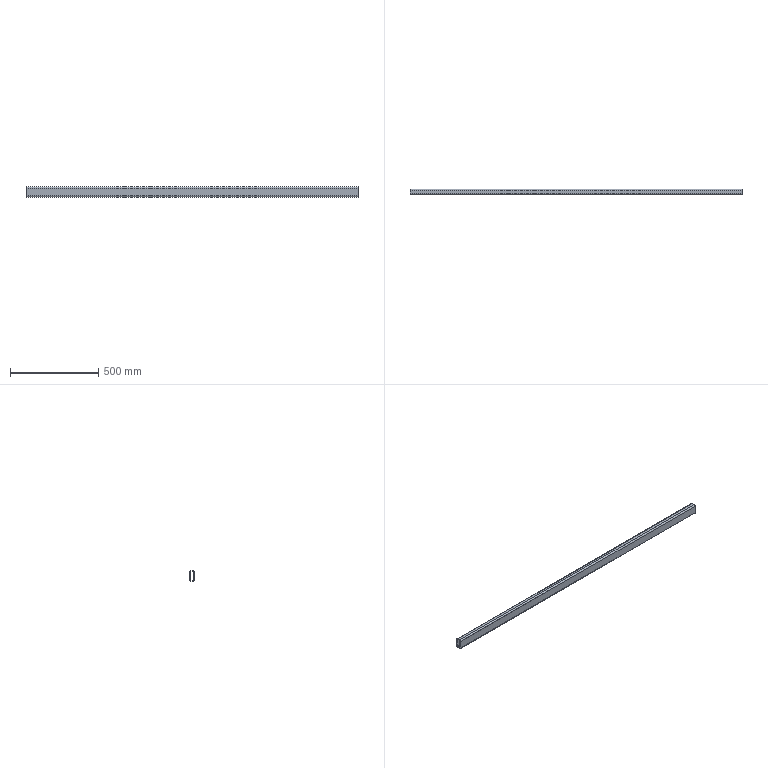Part | STEP file | 02-Rectangular tube 60x30x4_default<machining> | 1 solid | 18 faces | box 1880 x 30 x 60 mm | volume 1155817 mm3 | plane 10 | cylinder 8 | commonest cylinder face diameters 8 x4 16 x4
STEP:
#1=CARTESIAN_POINT('',(0.,0.,0.));
#2=DIRECTION('',(0.,0.,1.));
#3=DIRECTION('',(1.,0.,0.));
#4=AXIS2_PLACEMENT_3D('',#1,#2,#3);
#5=CARTESIAN_POINT('',(0.,15.,22.));
#6=VERTEX_POINT('',#5);
#7=CARTESIAN_POINT('',(0.,7.,30.));
#8=VERTEX_POINT('',#7);
#9=CARTESIAN_POINT('',(0.,7.,22.));
#10=DIRECTION('',(1.,0.,0.));
#11=DIRECTION('',(0.,0.,-1.));
#12=AXIS2_PLACEMENT_3D('',#9,#10,#11);
#13=CIRCLE('',#12,8.);
#14=CARTESIAN_POINT('',(1880.,7.,22.));
#15=DIRECTION('',(-1.,0.,0.));
#16=DIRECTION('',(0.,0.,1.));
#17=AXIS2_PLACEMENT_3D('',#14,#15,#16);
#18=CYLINDRICAL_SURFACE('',#17,8.);
#19=CARTESIAN_POINT('',(3.142,1880.));
#20=DIRECTION('',(-1.,0.));
#21=VECTOR('',#20,1.);
#22=LINE('',#19,#21);
#23=(GEOMETRIC_REPRESENTATION_CONTEXT(2)PARAMETRIC_REPRESENTATION_CONTEXT()REPRESENTATION_CONTEXT('',''));
#24=DEFINITIONAL_REPRESENTATION('',(#22),#23);
#25=PCURVE('',#18,#24);
#26=CARTESIAN_POINT('',(0.,7.,22.));
#27=DIRECTION('',(1.,0.,0.));
#28=DIRECTION('',(0.,0.,-1.));
#29=AXIS2_PLACEMENT_3D('',#26,#27,#28);
#30=PLANE('',#29);
#31=CARTESIAN_POINT('',(0.,0.));
#32=DIRECTION('',(1.,0.));
#33=AXIS2_PLACEMENT_2D('',#31,#32);
#34=CIRCLE('',#33,8.);
#35=(GEOMETRIC_REPRESENTATION_CONTEXT(2)PARAMETRIC_REPRESENTATION_CONTEXT()REPRESENTATION_CONTEXT('',''));
#36=DEFINITIONAL_REPRESENTATION('',(#34),#35);
#37=PCURVE('',#30,#36);
#38=SURFACE_CURVE('',#13,(#25,#37),.PCURVE_S1.);
#39=EDGE_CURVE('',#6,#8,#38,.T.);
#40=ORIENTED_EDGE('',*,*,#39,.T.);
#41=CARTESIAN_POINT('',(1880.,7.,30.));
#42=VERTEX_POINT('',#41);
#43=CARTESIAN_POINT('',(1880.,7.,30.));
#44=DIRECTION('',(-1.,0.,0.));
#45=VECTOR('',#44,1.);
#46=LINE('',#43,#45);
#47=CARTESIAN_POINT('',(0.,0.));
#48=DIRECTION('',(0.,1.));
#49=VECTOR('',#48,1.);
#50=LINE('',#47,#49);
#51=(GEOMETRIC_REPRESENTATION_CONTEXT(2)PARAMETRIC_REPRESENTATION_CONTEXT()REPRESENTATION_CONTEXT('',''));
#52=DEFINITIONAL_REPRESENTATION('',(#50),#51);
#53=PCURVE('',#18,#52);
#54=CARTESIAN_POINT('',(1880.,7.,30.));
#55=DIRECTION('',(0.,0.,-1.));
#56=DIRECTION('',(-1.,0.,0.));
#57=AXIS2_PLACEMENT_3D('',#54,#55,#56);
#58=PLANE('',#57);
#59=CARTESIAN_POINT('',(0.,0.));
#60=DIRECTION('',(1.,0.));
#61=VECTOR('',#60,1.);
#62=LINE('',#59,#61);
#63=(GEOMETRIC_REPRESENTATION_CONTEXT(2)PARAMETRIC_REPRESENTATION_CONTEXT()REPRESENTATION_CONTEXT('',''));
#64=DEFINITIONAL_REPRESENTATION('',(#62),#63);
#65=PCURVE('',#58,#64);
#66=SURFACE_CURVE('',#46,(#53,#65),.PCURVE_S1.);
#67=EDGE_CURVE('',#42,#8,#66,.T.);
#68=ORIENTED_EDGE('',*,*,#67,.F.);
#69=CARTESIAN_POINT('',(1880.,15.,22.));
#70=VERTEX_POINT('',#69);
#71=CARTESIAN_POINT('',(1880.,7.,22.));
#72=DIRECTION('',(1.,0.,0.));
#73=DIRECTION('',(0.,0.,-1.));
#74=AXIS2_PLACEMENT_3D('',#71,#72,#73);
#75=CIRCLE('',#74,8.);
#76=CARTESIAN_POINT('',(3.142,0.));
#77=DIRECTION('',(-1.,0.));
#78=VECTOR('',#77,1.);
#79=LINE('',#76,#78);
#80=(GEOMETRIC_REPRESENTATION_CONTEXT(2)PARAMETRIC_REPRESENTATION_CONTEXT()REPRESENTATION_CONTEXT('',''));
#81=DEFINITIONAL_REPRESENTATION('',(#79),#80);
#82=PCURVE('',#18,#81);
#83=CARTESIAN_POINT('',(1880.,7.,22.));
#84=DIRECTION('',(1.,0.,0.));
#85=DIRECTION('',(0.,0.,-1.));
#86=AXIS2_PLACEMENT_3D('',#83,#84,#85);
#87=PLANE('',#86);
#88=CARTESIAN_POINT('',(0.,0.));
#89=DIRECTION('',(1.,0.));
#90=AXIS2_PLACEMENT_2D('',#88,#89);
#91=CIRCLE('',#90,8.);
#92=(GEOMETRIC_REPRESENTATION_CONTEXT(2)PARAMETRIC_REPRESENTATION_CONTEXT()REPRESENTATION_CONTEXT('',''));
#93=DEFINITIONAL_REPRESENTATION('',(#91),#92);
#94=PCURVE('',#87,#93);
#95=SURFACE_CURVE('',#75,(#82,#94),.PCURVE_S1.);
#96=EDGE_CURVE('',#70,#42,#95,.T.);
#97=ORIENTED_EDGE('',*,*,#96,.F.);
#98=CARTESIAN_POINT('',(1880.,15.,22.));
#99=DIRECTION('',(-1.,0.,0.));
#100=VECTOR('',#99,1.);
#101=LINE('',#98,#100);
#102=CARTESIAN_POINT('',(1.571,0.));
#103=DIRECTION('',(0.,1.));
#104=VECTOR('',#103,1.);
#105=LINE('',#102,#104);
#106=(GEOMETRIC_REPRESENTATION_CONTEXT(2)PARAMETRIC_REPRESENTATION_CONTEXT()REPRESENTATION_CONTEXT('',''));
#107=DEFINITIONAL_REPRESENTATION('',(#105),#106);
#108=PCURVE('',#18,#107);
#109=CARTESIAN_POINT('',(1880.,15.,22.));
#110=DIRECTION('',(0.,-1.,0.));
#111=DIRECTION('',(0.,0.,-1.));
#112=AXIS2_PLACEMENT_3D('',#109,#110,#111);
#113=PLANE('',#112);
#114=CARTESIAN_POINT('',(0.,0.));
#115=DIRECTION('',(0.,-1.));
#116=VECTOR('',#115,1.);
#117=LINE('',#114,#116);
#118=(GEOMETRIC_REPRESENTATION_CONTEXT(2)PARAMETRIC_REPRESENTATION_CONTEXT()REPRESENTATION_CONTEXT('',''));
#119=DEFINITIONAL_REPRESENTATION('',(#117),#118);
#120=PCURVE('',#113,#119);
#121=SURFACE_CURVE('',#101,(#108,#120),.PCURVE_S1.);
#122=EDGE_CURVE('',#70,#6,#121,.T.);
#123=ORIENTED_EDGE('',*,*,#122,.T.);
#124=EDGE_LOOP('',(#40,#68,#97,#123));
#125=FACE_BOUND('',#124,.T.);
#126=ADVANCED_FACE('',(#125),#18,.T.);
#127=CARTESIAN_POINT('',(0.,-7.,30.));
#128=VERTEX_POINT('',#127);
#129=CARTESIAN_POINT('',(0.,7.,30.));
#130=DIRECTION('',(0.,-1.,0.));
#131=VECTOR('',#130,1.);
#132=LINE('',#129,#131);
#133=CARTESIAN_POINT('',(1880.,0.));
#134=DIRECTION('',(0.,-1.));
#135=VECTOR('',#134,1.);
#136=LINE('',#133,#135);
#137=(GEOMETRIC_REPRESENTATION_CONTEXT(2)PARAMETRIC_REPRESENTATION_CONTEXT()REPRESENTATION_CONTEXT('',''));
#138=DEFINITIONAL_REPRESENTATION('',(#136),#137);
#139=PCURVE('',#58,#138);
#140=CARTESIAN_POINT('',(-8.,0.));
#141=DIRECTION('',(0.,-1.));
#142=VECTOR('',#141,1.);
#143=LINE('',#140,#142);
#144=(GEOMETRIC_REPRESENTATION_CONTEXT(2)PARAMETRIC_REPRESENTATION_CONTEXT()REPRESENTATION_CONTEXT('',''));
#145=DEFINITIONAL_REPRESENTATION('',(#143),#144);
#146=PCURVE('',#30,#145);
#147=SURFACE_CURVE('',#132,(#139,#146),.PCURVE_S1.);
#148=EDGE_CURVE('',#8,#128,#147,.T.);
#149=ORIENTED_EDGE('',*,*,#148,.T.);
#150=CARTESIAN_POINT('',(1880.,-7.,30.));
#151=VERTEX_POINT('',#150);
#152=CARTESIAN_POINT('',(1880.,-7.,30.));
#153=DIRECTION('',(-1.,0.,0.));
#154=VECTOR('',#153,1.);
#155=LINE('',#152,#154);
#156=CARTESIAN_POINT('',(0.,-14.));
#157=DIRECTION('',(1.,0.));
#158=VECTOR('',#157,1.);
#159=LINE('',#156,#158);
#160=(GEOMETRIC_REPRESENTATION_CONTEXT(2)PARAMETRIC_REPRESENTATION_CONTEXT()REPRESENTATION_CONTEXT('',''));
#161=DEFINITIONAL_REPRESENTATION('',(#159),#160);
#162=PCURVE('',#58,#161);
#163=CARTESIAN_POINT('',(1880.,-7.,22.));
#164=DIRECTION('',(-1.,0.,0.));
#165=DIRECTION('',(0.,0.,1.));
#166=AXIS2_PLACEMENT_3D('',#163,#164,#165);
#167=CYLINDRICAL_SURFACE('',#166,8.);
#168=CARTESIAN_POINT('',(6.283,0.));
#169=DIRECTION('',(0.,1.));
#170=VECTOR('',#169,1.);
#171=LINE('',#168,#170);
#172=(GEOMETRIC_REPRESENTATION_CONTEXT(2)PARAMETRIC_REPRESENTATION_CONTEXT()REPRESENTATION_CONTEXT('',''));
#173=DEFINITIONAL_REPRESENTATION('',(#171),#172);
#174=PCURVE('',#167,#173);
#175=SURFACE_CURVE('',#155,(#162,#174),.PCURVE_S1.);
#176=EDGE_CURVE('',#151,#128,#175,.T.);
#177=ORIENTED_EDGE('',*,*,#176,.F.);
#178=CARTESIAN_POINT('',(1880.,7.,30.));
#179=DIRECTION('',(0.,-1.,0.));
#180=VECTOR('',#179,1.);
#181=LINE('',#178,#180);
#182=CARTESIAN_POINT('',(0.,0.));
#183=DIRECTION('',(0.,-1.));
#184=VECTOR('',#183,1.);
#185=LINE('',#182,#184);
#186=(GEOMETRIC_REPRESENTATION_CONTEXT(2)PARAMETRIC_REPRESENTATION_CONTEXT()REPRESENTATION_CONTEXT('',''));
#187=DEFINITIONAL_REPRESENTATION('',(#185),#186);
#188=PCURVE('',#58,#187);
#189=CARTESIAN_POINT('',(-8.,0.));
#190=DIRECTION('',(0.,-1.));
#191=VECTOR('',#190,1.);
#192=LINE('',#189,#191);
#193=(GEOMETRIC_REPRESENTATION_CONTEXT(2)PARAMETRIC_REPRESENTATION_CONTEXT()REPRESENTATION_CONTEXT('',''));
#194=DEFINITIONAL_REPRESENTATION('',(#192),#193);
#195=PCURVE('',#87,#194);
#196=SURFACE_CURVE('',#181,(#188,#195),.PCURVE_S1.);
#197=EDGE_CURVE('',#42,#151,#196,.T.);
#198=ORIENTED_EDGE('',*,*,#197,.F.);
#199=ORIENTED_EDGE('',*,*,#67,.T.);
#200=EDGE_LOOP('',(#149,#177,#198,#199));
#201=FACE_BOUND('',#200,.T.);
#202=ADVANCED_FACE('',(#201),#58,.F.);
#203=CARTESIAN_POINT('',(0.,-15.,22.));
#204=VERTEX_POINT('',#203);
#205=CARTESIAN_POINT('',(0.,-7.,22.));
#206=DIRECTION('',(1.,0.,0.));
#207=DIRECTION('',(0.,0.,-1.));
#208=AXIS2_PLACEMENT_3D('',#205,#206,#207);
#209=CIRCLE('',#208,8.);
#210=CARTESIAN_POINT('',(9.425,1880.));
#211=DIRECTION('',(-1.,0.));
#212=VECTOR('',#211,1.);
#213=LINE('',#210,#212);
#214=(GEOMETRIC_REPRESENTATION_CONTEXT(2)PARAMETRIC_REPRESENTATION_CONTEXT()REPRESENTATION_CONTEXT('',''));
#215=DEFINITIONAL_REPRESENTATION('',(#213),#214);
#216=PCURVE('',#167,#215);
#217=CARTESIAN_POINT('',(0.,-14.));
#218=DIRECTION('',(1.,0.));
#219=AXIS2_PLACEMENT_2D('',#217,#218);
#220=CIRCLE('',#219,8.);
#221=(GEOMETRIC_REPRESENTATION_CONTEXT(2)PARAMETRIC_REPRESENTATION_CONTEXT()REPRESENTATION_CONTEXT('',''));
#222=DEFINITIONAL_REPRESENTATION('',(#220),#221);
#223=PCURVE('',#30,#222);
#224=SURFACE_CURVE('',#209,(#216,#223),.PCURVE_S1.);
#225=EDGE_CURVE('',#128,#204,#224,.T.);
#226=ORIENTED_EDGE('',*,*,#225,.T.);
#227=CARTESIAN_POINT('',(1880.,-15.,22.));
#228=VERTEX_POINT('',#227);
#229=CARTESIAN_POINT('',(1880.,-15.,22.));
#230=DIRECTION('',(-1.,0.,0.));
#231=VECTOR('',#230,1.);
#232=LINE('',#229,#231);
#233=CARTESIAN_POINT('',(4.712,0.));
#234=DIRECTION('',(0.,1.));
#235=VECTOR('',#234,1.);
#236=LINE('',#233,#235);
#237=(GEOMETRIC_REPRESENTATION_CONTEXT(2)PARAMETRIC_REPRESENTATION_CONTEXT()REPRESENTATION_CONTEXT('',''));
#238=DEFINITIONAL_REPRESENTATION('',(#236),#237);
#239=PCURVE('',#167,#238);
#240=CARTESIAN_POINT('',(1880.,-15.,-22.));
#241=DIRECTION('',(0.,1.,0.));
#242=DIRECTION('',(0.,0.,1.));
#243=AXIS2_PLACEMENT_3D('',#240,#241,#242);
#244=PLANE('',#243);
#245=CARTESIAN_POINT('',(44.,0.));
#246=DIRECTION('',(0.,-1.));
#247=VECTOR('',#246,1.);
#248=LINE('',#245,#247);
#249=(GEOMETRIC_REPRESENTATION_CONTEXT(2)PARAMETRIC_REPRESENTATION_CONTEXT()REPRESENTATION_CONTEXT('',''));
#250=DEFINITIONAL_REPRESENTATION('',(#248),#249);
#251=PCURVE('',#244,#250);
#252=SURFACE_CURVE('',#232,(#239,#251),.PCURVE_S1.);
#253=EDGE_CURVE('',#228,#204,#252,.T.);
#254=ORIENTED_EDGE('',*,*,#253,.F.);
#255=CARTESIAN_POINT('',(1880.,-7.,22.));
#256=DIRECTION('',(1.,0.,0.));
#257=DIRECTION('',(0.,0.,-1.));
#258=AXIS2_PLACEMENT_3D('',#255,#256,#257);
#259=CIRCLE('',#258,8.);
#260=CARTESIAN_POINT('',(9.425,0.));
#261=DIRECTION('',(-1.,0.));
#262=VECTOR('',#261,1.);
#263=LINE('',#260,#262);
#264=(GEOMETRIC_REPRESENTATION_CONTEXT(2)PARAMETRIC_REPRESENTATION_CONTEXT()REPRESENTATION_CONTEXT('',''));
#265=DEFINITIONAL_REPRESENTATION('',(#263),#264);
#266=PCURVE('',#167,#265);
#267=CARTESIAN_POINT('',(0.,-14.));
#268=DIRECTION('',(1.,0.));
#269=AXIS2_PLACEMENT_2D('',#267,#268);
#270=CIRCLE('',#269,8.);
#271=(GEOMETRIC_REPRESENTATION_CONTEXT(2)PARAMETRIC_REPRESENTATION_CONTEXT()REPRESENTATION_CONTEXT('',''));
#272=DEFINITIONAL_REPRESENTATION('',(#270),#271);
#273=PCURVE('',#87,#272);
#274=SURFACE_CURVE('',#259,(#266,#273),.PCURVE_S1.);
#275=EDGE_CURVE('',#151,#228,#274,.T.);
#276=ORIENTED_EDGE('',*,*,#275,.F.);
#277=ORIENTED_EDGE('',*,*,#176,.T.);
#278=EDGE_LOOP('',(#226,#254,#276,#277));
#279=FACE_BOUND('',#278,.T.);
#280=ADVANCED_FACE('',(#279),#167,.T.);
#281=CARTESIAN_POINT('',(0.,-15.,-22.));
#282=VERTEX_POINT('',#281);
#283=CARTESIAN_POINT('',(0.,-15.,-22.));
#284=DIRECTION('',(0.,0.,-1.));
#285=VECTOR('',#284,1.);
#286=LINE('',#283,#285);
#287=CARTESIAN_POINT('',(0.,-1880.));
#288=DIRECTION('',(-1.,0.));
#289=VECTOR('',#288,1.);
#290=LINE('',#287,#289);
#291=(GEOMETRIC_REPRESENTATION_CONTEXT(2)PARAMETRIC_REPRESENTATION_CONTEXT()REPRESENTATION_CONTEXT('',''));
#292=DEFINITIONAL_REPRESENTATION('',(#290),#291);
#293=PCURVE('',#244,#292);
#294=CARTESIAN_POINT('',(44.,-22.));
#295=DIRECTION('',(1.,0.));
#296=VECTOR('',#295,1.);
#297=LINE('',#294,#296);
#298=(GEOMETRIC_REPRESENTATION_CONTEXT(2)PARAMETRIC_REPRESENTATION_CONTEXT()REPRESENTATION_CONTEXT('',''));
#299=DEFINITIONAL_REPRESENTATION('',(#297),#298);
#300=PCURVE('',#30,#299);
#301=SURFACE_CURVE('',#286,(#293,#300),.PCURVE_S1.);
#302=EDGE_CURVE('',#204,#282,#301,.T.);
#303=ORIENTED_EDGE('',*,*,#302,.T.);
#304=CARTESIAN_POINT('',(1880.,-15.,-22.));
#305=VERTEX_POINT('',#304);
#306=CARTESIAN_POINT('',(1880.,-15.,-22.));
#307=DIRECTION('',(-1.,0.,0.));
#308=VECTOR('',#307,1.);
#309=LINE('',#306,#308);
#310=CARTESIAN_POINT('',(0.,0.));
#311=DIRECTION('',(0.,-1.));
#312=VECTOR('',#311,1.);
#313=LINE('',#310,#312);
#314=(GEOMETRIC_REPRESENTATION_CONTEXT(2)PARAMETRIC_REPRESENTATION_CONTEXT()REPRESENTATION_CONTEXT('',''));
#315=DEFINITIONAL_REPRESENTATION('',(#313),#314);
#316=PCURVE('',#244,#315);
#317=CARTESIAN_POINT('',(1880.,-7.,-22.));
#318=DIRECTION('',(-1.,0.,0.));
#319=DIRECTION('',(0.,0.,1.));
#320=AXIS2_PLACEMENT_3D('',#317,#318,#319);
#321=CYLINDRICAL_SURFACE('',#320,8.);
#322=CARTESIAN_POINT('',(4.712,0.));
#323=DIRECTION('',(0.,1.));
#324=VECTOR('',#323,1.);
#325=LINE('',#322,#324);
#326=(GEOMETRIC_REPRESENTATION_CONTEXT(2)PARAMETRIC_REPRESENTATION_CONTEXT()REPRESENTATION_CONTEXT('',''));
#327=DEFINITIONAL_REPRESENTATION('',(#325),#326);
#328=PCURVE('',#321,#327);
#329=SURFACE_CURVE('',#309,(#316,#328),.PCURVE_S1.);
#330=EDGE_CURVE('',#305,#282,#329,.T.);
#331=ORIENTED_EDGE('',*,*,#330,.F.);
#332=CARTESIAN_POINT('',(1880.,-15.,-22.));
#333=DIRECTION('',(0.,0.,-1.));
#334=VECTOR('',#333,1.);
#335=LINE('',#332,#334);
#336=CARTESIAN_POINT('',(0.,0.));
#337=DIRECTION('',(-1.,0.));
#338=VECTOR('',#337,1.);
#339=LINE('',#336,#338);
#340=(GEOMETRIC_REPRESENTATION_CONTEXT(2)PARAMETRIC_REPRESENTATION_CONTEXT()REPRESENTATION_CONTEXT('',''));
#341=DEFINITIONAL_REPRESENTATION('',(#339),#340);
#342=PCURVE('',#244,#341);
#343=CARTESIAN_POINT('',(44.,-22.));
#344=DIRECTION('',(1.,0.));
#345=VECTOR('',#344,1.);
#346=LINE('',#343,#345);
#347=(GEOMETRIC_REPRESENTATION_CONTEXT(2)PARAMETRIC_REPRESENTATION_CONTEXT()REPRESENTATION_CONTEXT('',''));
#348=DEFINITIONAL_REPRESENTATION('',(#346),#347);
#349=PCURVE('',#87,#348);
#350=SURFACE_CURVE('',#335,(#342,#349),.PCURVE_S1.);
#351=EDGE_CURVE('',#228,#305,#350,.T.);
#352=ORIENTED_EDGE('',*,*,#351,.F.);
#353=ORIENTED_EDGE('',*,*,#253,.T.);
#354=EDGE_LOOP('',(#303,#331,#352,#353));
#355=FACE_BOUND('',#354,.T.);
#356=ADVANCED_FACE('',(#355),#244,.F.);
#357=CARTESIAN_POINT('',(0.,-7.,-30.));
#358=VERTEX_POINT('',#357);
#359=CARTESIAN_POINT('',(0.,-7.,-22.));
#360=DIRECTION('',(1.,0.,0.));
#361=DIRECTION('',(0.,0.,-1.));
#362=AXIS2_PLACEMENT_3D('',#359,#360,#361);
#363=CIRCLE('',#362,8.);
#364=CARTESIAN_POINT('',(9.425,1880.));
#365=DIRECTION('',(-1.,0.));
#366=VECTOR('',#365,1.);
#367=LINE('',#364,#366);
#368=(GEOMETRIC_REPRESENTATION_CONTEXT(2)PARAMETRIC_REPRESENTATION_CONTEXT()REPRESENTATION_CONTEXT('',''));
#369=DEFINITIONAL_REPRESENTATION('',(#367),#368);
#370=PCURVE('',#321,#369);
#371=CARTESIAN_POINT('',(44.,-14.));
#372=DIRECTION('',(1.,0.));
#373=AXIS2_PLACEMENT_2D('',#371,#372);
#374=CIRCLE('',#373,8.);
#375=(GEOMETRIC_REPRESENTATION_CONTEXT(2)PARAMETRIC_REPRESENTATION_CONTEXT()REPRESENTATION_CONTEXT('',''));
#376=DEFINITIONAL_REPRESENTATION('',(#374),#375);
#377=PCURVE('',#30,#376);
#378=SURFACE_CURVE('',#363,(#370,#377),.PCURVE_S1.);
#379=EDGE_CURVE('',#282,#358,#378,.T.);
#380=ORIENTED_EDGE('',*,*,#379,.T.);
#381=CARTESIAN_POINT('',(1880.,-7.,-30.));
#382=VERTEX_POINT('',#381);
#383=CARTESIAN_POINT('',(1880.,-7.,-30.));
#384=DIRECTION('',(-1.,0.,0.));
#385=VECTOR('',#384,1.);
#386=LINE('',#383,#385);
#387=CARTESIAN_POINT('',(3.142,0.));
#388=DIRECTION('',(0.,1.));
#389=VECTOR('',#388,1.);
#390=LINE('',#387,#389);
#391=(GEOMETRIC_REPRESENTATION_CONTEXT(2)PARAMETRIC_REPRESENTATION_CONTEXT()REPRESENTATION_CONTEXT('',''));
#392=DEFINITIONAL_REPRESENTATION('',(#390),#391);
#393=PCURVE('',#321,#392);
#394=CARTESIAN_POINT('',(1880.,-7.,-30.));
#395=DIRECTION('',(0.,0.,1.));
#396=DIRECTION('',(1.,0.,0.));
#397=AXIS2_PLACEMENT_3D('',#394,#395,#396);
#398=PLANE('',#397);
#399=CARTESIAN_POINT('',(0.,0.));
#400=DIRECTION('',(-1.,0.));
#401=VECTOR('',#400,1.);
#402=LINE('',#399,#401);
#403=(GEOMETRIC_REPRESENTATION_CONTEXT(2)PARAMETRIC_REPRESENTATION_CONTEXT()REPRESENTATION_CONTEXT('',''));
#404=DEFINITIONAL_REPRESENTATION('',(#402),#403);
#405=PCURVE('',#398,#404);
#406=SURFACE_CURVE('',#386,(#393,#405),.PCURVE_S1.);
#407=EDGE_CURVE('',#382,#358,#406,.T.);
#408=ORIENTED_EDGE('',*,*,#407,.F.);
#409=CARTESIAN_POINT('',(1880.,-7.,-22.));
#410=DIRECTION('',(1.,0.,0.));
#411=DIRECTION('',(0.,0.,-1.));
#412=AXIS2_PLACEMENT_3D('',#409,#410,#411);
#413=CIRCLE('',#412,8.);
#414=CARTESIAN_POINT('',(9.425,0.));
#415=DIRECTION('',(-1.,0.));
#416=VECTOR('',#415,1.);
#417=LINE('',#414,#416);
#418=(GEOMETRIC_REPRESENTATION_CONTEXT(2)PARAMETRIC_REPRESENTATION_CONTEXT()REPRESENTATION_CONTEXT('',''));
#419=DEFINITIONAL_REPRESENTATION('',(#417),#418);
#420=PCURVE('',#321,#419);
#421=CARTESIAN_POINT('',(44.,-14.));
#422=DIRECTION('',(1.,0.));
#423=AXIS2_PLACEMENT_2D('',#421,#422);
#424=CIRCLE('',#423,8.);
#425=(GEOMETRIC_REPRESENTATION_CONTEXT(2)PARAMETRIC_REPRESENTATION_CONTEXT()REPRESENTATION_CONTEXT('',''));
#426=DEFINITIONAL_REPRESENTATION('',(#424),#425);
#427=PCURVE('',#87,#426);
#428=SURFACE_CURVE('',#413,(#420,#427),.PCURVE_S1.);
#429=EDGE_CURVE('',#305,#382,#428,.T.);
#430=ORIENTED_EDGE('',*,*,#429,.F.);
#431=ORIENTED_EDGE('',*,*,#330,.T.);
#432=EDGE_LOOP('',(#380,#408,#430,#431));
#433=FACE_BOUND('',#432,.T.);
#434=ADVANCED_FACE('',(#433),#321,.T.);
#435=CARTESIAN_POINT('',(0.,7.,-30.));
#436=VERTEX_POINT('',#435);
#437=CARTESIAN_POINT('',(0.,-7.,-30.));
#438=DIRECTION('',(0.,1.,0.));
#439=VECTOR('',#438,1.);
#440=LINE('',#437,#439);
#441=CARTESIAN_POINT('',(-1880.,0.));
#442=DIRECTION('',(0.,1.));
#443=VECTOR('',#442,1.);
#444=LINE('',#441,#443);
#445=(GEOMETRIC_REPRESENTATION_CONTEXT(2)PARAMETRIC_REPRESENTATION_CONTEXT()REPRESENTATION_CONTEXT('',''));
#446=DEFINITIONAL_REPRESENTATION('',(#444),#445);
#447=PCURVE('',#398,#446);
#448=CARTESIAN_POINT('',(52.,-14.));
#449=DIRECTION('',(0.,1.));
#450=VECTOR('',#449,1.);
#451=LINE('',#448,#450);
#452=(GEOMETRIC_REPRESENTATION_CONTEXT(2)PARAMETRIC_REPRESENTATION_CONTEXT()REPRESENTATION_CONTEXT('',''));
#453=DEFINITIONAL_REPRESENTATION('',(#451),#452);
#454=PCURVE('',#30,#453);
#455=SURFACE_CURVE('',#440,(#447,#454),.PCURVE_S1.);
#456=EDGE_CURVE('',#358,#436,#455,.T.);
#457=ORIENTED_EDGE('',*,*,#456,.T.);
#458=CARTESIAN_POINT('',(1880.,7.,-30.));
#459=VERTEX_POINT('',#458);
#460=CARTESIAN_POINT('',(1880.,7.,-30.));
#461=DIRECTION('',(-1.,0.,0.));
#462=VECTOR('',#461,1.);
#463=LINE('',#460,#462);
#464=CARTESIAN_POINT('',(0.,14.));
#465=DIRECTION('',(-1.,0.));
#466=VECTOR('',#465,1.);
#467=LINE('',#464,#466);
#468=(GEOMETRIC_REPRESENTATION_CONTEXT(2)PARAMETRIC_REPRESENTATION_CONTEXT()REPRESENTATION_CONTEXT('',''));
#469=DEFINITIONAL_REPRESENTATION('',(#467),#468);
#470=PCURVE('',#398,#469);
#471=CARTESIAN_POINT('',(1880.,7.,-22.));
#472=DIRECTION('',(-1.,0.,0.));
#473=DIRECTION('',(0.,0.,1.));
#474=AXIS2_PLACEMENT_3D('',#471,#472,#473);
#475=CYLINDRICAL_SURFACE('',#474,8.);
#476=CARTESIAN_POINT('',(3.142,0.));
#477=DIRECTION('',(0.,1.));
#478=VECTOR('',#477,1.);
#479=LINE('',#476,#478);
#480=(GEOMETRIC_REPRESENTATION_CONTEXT(2)PARAMETRIC_REPRESENTATION_CONTEXT()REPRESENTATION_CONTEXT('',''));
#481=DEFINITIONAL_REPRESENTATION('',(#479),#480);
#482=PCURVE('',#475,#481);
#483=SURFACE_CURVE('',#463,(#470,#482),.PCURVE_S1.);
#484=EDGE_CURVE('',#459,#436,#483,.T.);
#485=ORIENTED_EDGE('',*,*,#484,.F.);
#486=CARTESIAN_POINT('',(1880.,-7.,-30.));
#487=DIRECTION('',(0.,1.,0.));
#488=VECTOR('',#487,1.);
#489=LINE('',#486,#488);
#490=CARTESIAN_POINT('',(0.,0.));
#491=DIRECTION('',(0.,1.));
#492=VECTOR('',#491,1.);
#493=LINE('',#490,#492);
#494=(GEOMETRIC_REPRESENTATION_CONTEXT(2)PARAMETRIC_REPRESENTATION_CONTEXT()REPRESENTATION_CONTEXT('',''));
#495=DEFINITIONAL_REPRESENTATION('',(#493),#494);
#496=PCURVE('',#398,#495);
#497=CARTESIAN_POINT('',(52.,-14.));
#498=DIRECTION('',(0.,1.));
#499=VECTOR('',#498,1.);
#500=LINE('',#497,#499);
#501=(GEOMETRIC_REPRESENTATION_CONTEXT(2)PARAMETRIC_REPRESENTATION_CONTEXT()REPRESENTATION_CONTEXT('',''));
#502=DEFINITIONAL_REPRESENTATION('',(#500),#501);
#503=PCURVE('',#87,#502);
#504=SURFACE_CURVE('',#489,(#496,#503),.PCURVE_S1.);
#505=EDGE_CURVE('',#382,#459,#504,.T.);
#506=ORIENTED_EDGE('',*,*,#505,.F.);
#507=ORIENTED_EDGE('',*,*,#407,.T.);
#508=EDGE_LOOP('',(#457,#485,#506,#507));
#509=FACE_BOUND('',#508,.T.);
#510=ADVANCED_FACE('',(#509),#398,.F.);
#511=CARTESIAN_POINT('',(0.,15.,-22.));
#512=VERTEX_POINT('',#511);
#513=CARTESIAN_POINT('',(0.,7.,-22.));
#514=DIRECTION('',(1.,0.,0.));
#515=DIRECTION('',(0.,0.,-1.));
#516=AXIS2_PLACEMENT_3D('',#513,#514,#515);
#517=CIRCLE('',#516,8.);
#518=CARTESIAN_POINT('',(3.142,1880.));
#519=DIRECTION('',(-1.,0.));
#520=VECTOR('',#519,1.);
#521=LINE('',#518,#520);
#522=(GEOMETRIC_REPRESENTATION_CONTEXT(2)PARAMETRIC_REPRESENTATION_CONTEXT()REPRESENTATION_CONTEXT('',''));
#523=DEFINITIONAL_REPRESENTATION('',(#521),#522);
#524=PCURVE('',#475,#523);
#525=CARTESIAN_POINT('',(44.,0.));
#526=DIRECTION('',(1.,0.));
#527=AXIS2_PLACEMENT_2D('',#525,#526);
#528=CIRCLE('',#527,8.);
#529=(GEOMETRIC_REPRESENTATION_CONTEXT(2)PARAMETRIC_REPRESENTATION_CONTEXT()REPRESENTATION_CONTEXT('',''));
#530=DEFINITIONAL_REPRESENTATION('',(#528),#529);
#531=PCURVE('',#30,#530);
#532=SURFACE_CURVE('',#517,(#524,#531),.PCURVE_S1.);
#533=EDGE_CURVE('',#436,#512,#532,.T.);
#534=ORIENTED_EDGE('',*,*,#533,.T.);
#535=CARTESIAN_POINT('',(1880.,15.,-22.));
#536=VERTEX_POINT('',#535);
#537=CARTESIAN_POINT('',(1880.,15.,-22.));
#538=DIRECTION('',(-1.,0.,0.));
#539=VECTOR('',#538,1.);
#540=LINE('',#537,#539);
#541=CARTESIAN_POINT('',(1.571,0.));
#542=DIRECTION('',(0.,1.));
#543=VECTOR('',#542,1.);
#544=LINE('',#541,#543);
#545=(GEOMETRIC_REPRESENTATION_CONTEXT(2)PARAMETRIC_REPRESENTATION_CONTEXT()REPRESENTATION_CONTEXT('',''));
#546=DEFINITIONAL_REPRESENTATION('',(#544),#545);
#547=PCURVE('',#475,#546);
#548=CARTESIAN_POINT('',(44.,0.));
#549=DIRECTION('',(0.,-1.));
#550=VECTOR('',#549,1.);
#551=LINE('',#548,#550);
#552=(GEOMETRIC_REPRESENTATION_CONTEXT(2)PARAMETRIC_REPRESENTATION_CONTEXT()REPRESENTATION_CONTEXT('',''));
#553=DEFINITIONAL_REPRESENTATION('',(#551),#552);
#554=PCURVE('',#113,#553);
#555=SURFACE_CURVE('',#540,(#547,#554),.PCURVE_S1.);
#556=EDGE_CURVE('',#536,#512,#555,.T.);
#557=ORIENTED_EDGE('',*,*,#556,.F.);
#558=CARTESIAN_POINT('',(1880.,7.,-22.));
#559=DIRECTION('',(1.,0.,0.));
#560=DIRECTION('',(0.,0.,-1.));
#561=AXIS2_PLACEMENT_3D('',#558,#559,#560);
#562=CIRCLE('',#561,8.);
#563=CARTESIAN_POINT('',(3.142,0.));
#564=DIRECTION('',(-1.,0.));
#565=VECTOR('',#564,1.);
#566=LINE('',#563,#565);
#567=(GEOMETRIC_REPRESENTATION_CONTEXT(2)PARAMETRIC_REPRESENTATION_CONTEXT()REPRESENTATION_CONTEXT('',''));
#568=DEFINITIONAL_REPRESENTATION('',(#566),#567);
#569=PCURVE('',#475,#568);
#570=CARTESIAN_POINT('',(44.,0.));
#571=DIRECTION('',(1.,0.));
#572=AXIS2_PLACEMENT_2D('',#570,#571);
#573=CIRCLE('',#572,8.);
#574=(GEOMETRIC_REPRESENTATION_CONTEXT(2)PARAMETRIC_REPRESENTATION_CONTEXT()REPRESENTATION_CONTEXT('',''));
#575=DEFINITIONAL_REPRESENTATION('',(#573),#574);
#576=PCURVE('',#87,#575);
#577=SURFACE_CURVE('',#562,(#569,#576),.PCURVE_S1.);
#578=EDGE_CURVE('',#459,#536,#577,.T.);
#579=ORIENTED_EDGE('',*,*,#578,.F.);
#580=ORIENTED_EDGE('',*,*,#484,.T.);
#581=EDGE_LOOP('',(#534,#557,#579,#580));
#582=FACE_BOUND('',#581,.T.);
#583=ADVANCED_FACE('',(#582),#475,.T.);
#584=CARTESIAN_POINT('',(1880.,-11.,22.));
#585=VERTEX_POINT('',#584);
#586=CARTESIAN_POINT('',(0.,-11.,22.));
#587=VERTEX_POINT('',#586);
#588=CARTESIAN_POINT('',(1880.,-11.,22.));
#589=DIRECTION('',(-1.,0.,0.));
#590=VECTOR('',#589,1.);
#591=LINE('',#588,#590);
#592=CARTESIAN_POINT('',(1880.,-7.,22.));
#593=DIRECTION('',(-1.,0.,0.));
#594=DIRECTION('',(0.,0.,1.));
#595=AXIS2_PLACEMENT_3D('',#592,#593,#594);
#596=CYLINDRICAL_SURFACE('',#595,4.);
#597=CARTESIAN_POINT('',(4.712,0.));
#598=DIRECTION('',(0.,1.));
#599=VECTOR('',#598,1.);
#600=LINE('',#597,#599);
#601=(GEOMETRIC_REPRESENTATION_CONTEXT(2)PARAMETRIC_REPRESENTATION_CONTEXT()REPRESENTATION_CONTEXT('',''));
#602=DEFINITIONAL_REPRESENTATION('',(#600),#601);
#603=PCURVE('',#596,#602);
#604=CARTESIAN_POINT('',(1880.,-11.,-22.));
#605=DIRECTION('',(0.,1.,0.));
#606=DIRECTION('',(0.,0.,1.));
#607=AXIS2_PLACEMENT_3D('',#604,#605,#606);
#608=PLANE('',#607);
#609=CARTESIAN_POINT('',(44.,0.));
#610=DIRECTION('',(0.,-1.));
#611=VECTOR('',#610,1.);
#612=LINE('',#609,#611);
#613=(GEOMETRIC_REPRESENTATION_CONTEXT(2)PARAMETRIC_REPRESENTATION_CONTEXT()REPRESENTATION_CONTEXT('',''));
#614=DEFINITIONAL_REPRESENTATION('',(#612),#613);
#615=PCURVE('',#608,#614);
#616=SURFACE_CURVE('',#591,(#603,#615),.PCURVE_S1.);
#617=EDGE_CURVE('',#585,#587,#616,.T.);
#618=ORIENTED_EDGE('',*,*,#617,.F.);
#619=CARTESIAN_POINT('',(1880.,-7.,26.));
#620=VERTEX_POINT('',#619);
#621=CARTESIAN_POINT('',(1880.,-7.,22.));
#622=DIRECTION('',(1.,0.,0.));
#623=DIRECTION('',(0.,0.,-1.));
#624=AXIS2_PLACEMENT_3D('',#621,#622,#623);
#625=CIRCLE('',#624,4.);
#626=CARTESIAN_POINT('',(9.425,0.));
#627=DIRECTION('',(-1.,0.));
#628=VECTOR('',#627,1.);
#629=LINE('',#626,#628);
#630=(GEOMETRIC_REPRESENTATION_CONTEXT(2)PARAMETRIC_REPRESENTATION_CONTEXT()REPRESENTATION_CONTEXT('',''));
#631=DEFINITIONAL_REPRESENTATION('',(#629),#630);
#632=PCURVE('',#596,#631);
#633=CARTESIAN_POINT('',(0.,-14.));
#634=DIRECTION('',(1.,0.));
#635=AXIS2_PLACEMENT_2D('',#633,#634);
#636=CIRCLE('',#635,4.);
#637=(GEOMETRIC_REPRESENTATION_CONTEXT(2)PARAMETRIC_REPRESENTATION_CONTEXT()REPRESENTATION_CONTEXT('',''));
#638=DEFINITIONAL_REPRESENTATION('',(#636),#637);
#639=PCURVE('',#87,#638);
#640=SURFACE_CURVE('',#625,(#632,#639),.PCURVE_S1.);
#641=EDGE_CURVE('',#620,#585,#640,.T.);
#642=ORIENTED_EDGE('',*,*,#641,.F.);
#643=CARTESIAN_POINT('',(0.,-7.,26.));
#644=VERTEX_POINT('',#643);
#645=CARTESIAN_POINT('',(1880.,-7.,26.));
#646=DIRECTION('',(-1.,0.,0.));
#647=VECTOR('',#646,1.);
#648=LINE('',#645,#647);
#649=CARTESIAN_POINT('',(6.283,0.));
#650=DIRECTION('',(0.,1.));
#651=VECTOR('',#650,1.);
#652=LINE('',#649,#651);
#653=(GEOMETRIC_REPRESENTATION_CONTEXT(2)PARAMETRIC_REPRESENTATION_CONTEXT()REPRESENTATION_CONTEXT('',''));
#654=DEFINITIONAL_REPRESENTATION('',(#652),#653);
#655=PCURVE('',#596,#654);
#656=CARTESIAN_POINT('',(1880.,7.,26.));
#657=DIRECTION('',(0.,0.,-1.));
#658=DIRECTION('',(-1.,0.,0.));
#659=AXIS2_PLACEMENT_3D('',#656,#657,#658);
#660=PLANE('',#659);
#661=CARTESIAN_POINT('',(0.,-14.));
#662=DIRECTION('',(1.,0.));
#663=VECTOR('',#662,1.);
#664=LINE('',#661,#663);
#665=(GEOMETRIC_REPRESENTATION_CONTEXT(2)PARAMETRIC_REPRESENTATION_CONTEXT()REPRESENTATION_CONTEXT('',''));
#666=DEFINITIONAL_REPRESENTATION('',(#664),#665);
#667=PCURVE('',#660,#666);
#668=SURFACE_CURVE('',#648,(#655,#667),.PCURVE_S1.);
#669=EDGE_CURVE('',#620,#644,#668,.T.);
#670=ORIENTED_EDGE('',*,*,#669,.T.);
#671=CARTESIAN_POINT('',(0.,-7.,22.));
#672=DIRECTION('',(1.,0.,0.));
#673=DIRECTION('',(0.,0.,-1.));
#674=AXIS2_PLACEMENT_3D('',#671,#672,#673);
#675=CIRCLE('',#674,4.);
#676=CARTESIAN_POINT('',(9.425,1880.));
#677=DIRECTION('',(-1.,0.));
#678=VECTOR('',#677,1.);
#679=LINE('',#676,#678);
#680=(GEOMETRIC_REPRESENTATION_CONTEXT(2)PARAMETRIC_REPRESENTATION_CONTEXT()REPRESENTATION_CONTEXT('',''));
#681=DEFINITIONAL_REPRESENTATION('',(#679),#680);
#682=PCURVE('',#596,#681);
#683=CARTESIAN_POINT('',(0.,-14.));
#684=DIRECTION('',(1.,0.));
#685=AXIS2_PLACEMENT_2D('',#683,#684);
#686=CIRCLE('',#685,4.);
#687=(GEOMETRIC_REPRESENTATION_CONTEXT(2)PARAMETRIC_REPRESENTATION_CONTEXT()REPRESENTATION_CONTEXT('',''));
#688=DEFINITIONAL_REPRESENTATION('',(#686),#687);
#689=PCURVE('',#30,#688);
#690=SURFACE_CURVE('',#675,(#682,#689),.PCURVE_S1.);
#691=EDGE_CURVE('',#644,#587,#690,.T.);
#692=ORIENTED_EDGE('',*,*,#691,.T.);
#693=EDGE_LOOP('',(#618,#642,#670,#692));
#694=FACE_BOUND('',#693,.F.);
#695=ADVANCED_FACE('',(#694),#596,.F.);
#696=CARTESIAN_POINT('',(0.,7.,26.));
#697=VERTEX_POINT('',#696);
#698=CARTESIAN_POINT('',(0.,7.,26.));
#699=DIRECTION('',(0.,-1.,0.));
#700=VECTOR('',#699,1.);
#701=LINE('',#698,#700);
#702=CARTESIAN_POINT('',(1880.,0.));
#703=DIRECTION('',(0.,-1.));
#704=VECTOR('',#703,1.);
#705=LINE('',#702,#704);
#706=(GEOMETRIC_REPRESENTATION_CONTEXT(2)PARAMETRIC_REPRESENTATION_CONTEXT()REPRESENTATION_CONTEXT('',''));
#707=DEFINITIONAL_REPRESENTATION('',(#705),#706);
#708=PCURVE('',#660,#707);
#709=CARTESIAN_POINT('',(-4.,0.));
#710=DIRECTION('',(0.,-1.));
#711=VECTOR('',#710,1.);
#712=LINE('',#709,#711);
#713=(GEOMETRIC_REPRESENTATION_CONTEXT(2)PARAMETRIC_REPRESENTATION_CONTEXT()REPRESENTATION_CONTEXT('',''));
#714=DEFINITIONAL_REPRESENTATION('',(#712),#713);
#715=PCURVE('',#30,#714);
#716=SURFACE_CURVE('',#701,(#708,#715),.PCURVE_S1.);
#717=EDGE_CURVE('',#697,#644,#716,.T.);
#718=ORIENTED_EDGE('',*,*,#717,.F.);
#719=CARTESIAN_POINT('',(1880.,7.,26.));
#720=VERTEX_POINT('',#719);
#721=CARTESIAN_POINT('',(1880.,7.,26.));
#722=DIRECTION('',(-1.,0.,0.));
#723=VECTOR('',#722,1.);
#724=LINE('',#721,#723);
#725=CARTESIAN_POINT('',(0.,0.));
#726=DIRECTION('',(1.,0.));
#727=VECTOR('',#726,1.);
#728=LINE('',#725,#727);
#729=(GEOMETRIC_REPRESENTATION_CONTEXT(2)PARAMETRIC_REPRESENTATION_CONTEXT()REPRESENTATION_CONTEXT('',''));
#730=DEFINITIONAL_REPRESENTATION('',(#728),#729);
#731=PCURVE('',#660,#730);
#732=CARTESIAN_POINT('',(1880.,7.,22.));
#733=DIRECTION('',(-1.,0.,0.));
#734=DIRECTION('',(0.,0.,1.));
#735=AXIS2_PLACEMENT_3D('',#732,#733,#734);
#736=CYLINDRICAL_SURFACE('',#735,4.);
#737=CARTESIAN_POINT('',(0.,0.));
#738=DIRECTION('',(0.,1.));
#739=VECTOR('',#738,1.);
#740=LINE('',#737,#739);
#741=(GEOMETRIC_REPRESENTATION_CONTEXT(2)PARAMETRIC_REPRESENTATION_CONTEXT()REPRESENTATION_CONTEXT('',''));
#742=DEFINITIONAL_REPRESENTATION('',(#740),#741);
#743=PCURVE('',#736,#742);
#744=SURFACE_CURVE('',#724,(#731,#743),.PCURVE_S1.);
#745=EDGE_CURVE('',#720,#697,#744,.T.);
#746=ORIENTED_EDGE('',*,*,#745,.F.);
#747=CARTESIAN_POINT('',(1880.,7.,26.));
#748=DIRECTION('',(0.,-1.,0.));
#749=VECTOR('',#748,1.);
#750=LINE('',#747,#749);
#751=CARTESIAN_POINT('',(0.,0.));
#752=DIRECTION('',(0.,-1.));
#753=VECTOR('',#752,1.);
#754=LINE('',#751,#753);
#755=(GEOMETRIC_REPRESENTATION_CONTEXT(2)PARAMETRIC_REPRESENTATION_CONTEXT()REPRESENTATION_CONTEXT('',''));
#756=DEFINITIONAL_REPRESENTATION('',(#754),#755);
#757=PCURVE('',#660,#756);
#758=CARTESIAN_POINT('',(-4.,0.));
#759=DIRECTION('',(0.,-1.));
#760=VECTOR('',#759,1.);
#761=LINE('',#758,#760);
#762=(GEOMETRIC_REPRESENTATION_CONTEXT(2)PARAMETRIC_REPRESENTATION_CONTEXT()REPRESENTATION_CONTEXT('',''));
#763=DEFINITIONAL_REPRESENTATION('',(#761),#762);
#764=PCURVE('',#87,#763);
#765=SURFACE_CURVE('',#750,(#757,#764),.PCURVE_S1.);
#766=EDGE_CURVE('',#720,#620,#765,.T.);
#767=ORIENTED_EDGE('',*,*,#766,.T.);
#768=ORIENTED_EDGE('',*,*,#669,.T.);
#769=EDGE_LOOP('',(#718,#746,#767,#768));
#770=FACE_BOUND('',#769,.T.);
#771=ADVANCED_FACE('',(#770),#660,.T.);
#772=ORIENTED_EDGE('',*,*,#745,.F.);
#773=CARTESIAN_POINT('',(1880.,11.,22.));
#774=VERTEX_POINT('',#773);
#775=CARTESIAN_POINT('',(1880.,7.,22.));
#776=DIRECTION('',(1.,0.,0.));
#777=DIRECTION('',(0.,0.,-1.));
#778=AXIS2_PLACEMENT_3D('',#775,#776,#777);
#779=CIRCLE('',#778,4.);
#780=CARTESIAN_POINT('',(3.142,0.));
#781=DIRECTION('',(-1.,0.));
#782=VECTOR('',#781,1.);
#783=LINE('',#780,#782);
#784=(GEOMETRIC_REPRESENTATION_CONTEXT(2)PARAMETRIC_REPRESENTATION_CONTEXT()REPRESENTATION_CONTEXT('',''));
#785=DEFINITIONAL_REPRESENTATION('',(#783),#784);
#786=PCURVE('',#736,#785);
#787=CARTESIAN_POINT('',(0.,0.));
#788=DIRECTION('',(1.,0.));
#789=AXIS2_PLACEMENT_2D('',#787,#788);
#790=CIRCLE('',#789,4.);
#791=(GEOMETRIC_REPRESENTATION_CONTEXT(2)PARAMETRIC_REPRESENTATION_CONTEXT()REPRESENTATION_CONTEXT('',''));
#792=DEFINITIONAL_REPRESENTATION('',(#790),#791);
#793=PCURVE('',#87,#792);
#794=SURFACE_CURVE('',#779,(#786,#793),.PCURVE_S1.);
#795=EDGE_CURVE('',#774,#720,#794,.T.);
#796=ORIENTED_EDGE('',*,*,#795,.F.);
#797=CARTESIAN_POINT('',(0.,11.,22.));
#798=VERTEX_POINT('',#797);
#799=CARTESIAN_POINT('',(1880.,11.,22.));
#800=DIRECTION('',(-1.,0.,0.));
#801=VECTOR('',#800,1.);
#802=LINE('',#799,#801);
#803=CARTESIAN_POINT('',(1.571,0.));
#804=DIRECTION('',(0.,1.));
#805=VECTOR('',#804,1.);
#806=LINE('',#803,#805);
#807=(GEOMETRIC_REPRESENTATION_CONTEXT(2)PARAMETRIC_REPRESENTATION_CONTEXT()REPRESENTATION_CONTEXT('',''));
#808=DEFINITIONAL_REPRESENTATION('',(#806),#807);
#809=PCURVE('',#736,#808);
#810=CARTESIAN_POINT('',(1880.,11.,22.));
#811=DIRECTION('',(0.,-1.,0.));
#812=DIRECTION('',(0.,0.,-1.));
#813=AXIS2_PLACEMENT_3D('',#810,#811,#812);
#814=PLANE('',#813);
#815=CARTESIAN_POINT('',(0.,0.));
#816=DIRECTION('',(0.,-1.));
#817=VECTOR('',#816,1.);
#818=LINE('',#815,#817);
#819=(GEOMETRIC_REPRESENTATION_CONTEXT(2)PARAMETRIC_REPRESENTATION_CONTEXT()REPRESENTATION_CONTEXT('',''));
#820=DEFINITIONAL_REPRESENTATION('',(#818),#819);
#821=PCURVE('',#814,#820);
#822=SURFACE_CURVE('',#802,(#809,#821),.PCURVE_S1.);
#823=EDGE_CURVE('',#774,#798,#822,.T.);
#824=ORIENTED_EDGE('',*,*,#823,.T.);
#825=CARTESIAN_POINT('',(0.,7.,22.));
#826=DIRECTION('',(1.,0.,0.));
#827=DIRECTION('',(0.,0.,-1.));
#828=AXIS2_PLACEMENT_3D('',#825,#826,#827);
#829=CIRCLE('',#828,4.);
#830=CARTESIAN_POINT('',(3.142,1880.));
#831=DIRECTION('',(-1.,0.));
#832=VECTOR('',#831,1.);
#833=LINE('',#830,#832);
#834=(GEOMETRIC_REPRESENTATION_CONTEXT(2)PARAMETRIC_REPRESENTATION_CONTEXT()REPRESENTATION_CONTEXT('',''));
#835=DEFINITIONAL_REPRESENTATION('',(#833),#834);
#836=PCURVE('',#736,#835);
#837=CARTESIAN_POINT('',(0.,0.));
#838=DIRECTION('',(1.,0.));
#839=AXIS2_PLACEMENT_2D('',#837,#838);
#840=CIRCLE('',#839,4.);
#841=(GEOMETRIC_REPRESENTATION_CONTEXT(2)PARAMETRIC_REPRESENTATION_CONTEXT()REPRESENTATION_CONTEXT('',''));
#842=DEFINITIONAL_REPRESENTATION('',(#840),#841);
#843=PCURVE('',#30,#842);
#844=SURFACE_CURVE('',#829,(#836,#843),.PCURVE_S1.);
#845=EDGE_CURVE('',#798,#697,#844,.T.);
#846=ORIENTED_EDGE('',*,*,#845,.T.);
#847=EDGE_LOOP('',(#772,#796,#824,#846));
#848=FACE_BOUND('',#847,.F.);
#849=ADVANCED_FACE('',(#848),#736,.F.);
#850=CARTESIAN_POINT('',(0.,11.,-22.));
#851=VERTEX_POINT('',#850);
#852=CARTESIAN_POINT('',(0.,11.,22.));
#853=DIRECTION('',(0.,0.,1.));
#854=VECTOR('',#853,1.);
#855=LINE('',#852,#854);
#856=CARTESIAN_POINT('',(0.,-1880.));
#857=DIRECTION('',(-1.,0.));
#858=VECTOR('',#857,1.);
#859=LINE('',#856,#858);
#860=(GEOMETRIC_REPRESENTATION_CONTEXT(2)PARAMETRIC_REPRESENTATION_CONTEXT()REPRESENTATION_CONTEXT('',''));
#861=DEFINITIONAL_REPRESENTATION('',(#859),#860);
#862=PCURVE('',#814,#861);
#863=CARTESIAN_POINT('',(0.,4.));
#864=DIRECTION('',(-1.,0.));
#865=VECTOR('',#864,1.);
#866=LINE('',#863,#865);
#867=(GEOMETRIC_REPRESENTATION_CONTEXT(2)PARAMETRIC_REPRESENTATION_CONTEXT()REPRESENTATION_CONTEXT('',''));
#868=DEFINITIONAL_REPRESENTATION('',(#866),#867);
#869=PCURVE('',#30,#868);
#870=SURFACE_CURVE('',#855,(#862,#869),.PCURVE_S1.);
#871=EDGE_CURVE('',#851,#798,#870,.T.);
#872=ORIENTED_EDGE('',*,*,#871,.F.);
#873=CARTESIAN_POINT('',(1880.,11.,-22.));
#874=VERTEX_POINT('',#873);
#875=CARTESIAN_POINT('',(1880.,11.,-22.));
#876=DIRECTION('',(-1.,0.,0.));
#877=VECTOR('',#876,1.);
#878=LINE('',#875,#877);
#879=CARTESIAN_POINT('',(44.,0.));
#880=DIRECTION('',(0.,-1.));
#881=VECTOR('',#880,1.);
#882=LINE('',#879,#881);
#883=(GEOMETRIC_REPRESENTATION_CONTEXT(2)PARAMETRIC_REPRESENTATION_CONTEXT()REPRESENTATION_CONTEXT('',''));
#884=DEFINITIONAL_REPRESENTATION('',(#882),#883);
#885=PCURVE('',#814,#884);
#886=CARTESIAN_POINT('',(1880.,7.,-22.));
#887=DIRECTION('',(-1.,0.,0.));
#888=DIRECTION('',(0.,0.,1.));
#889=AXIS2_PLACEMENT_3D('',#886,#887,#888);
#890=CYLINDRICAL_SURFACE('',#889,4.);
#891=CARTESIAN_POINT('',(1.571,0.));
#892=DIRECTION('',(0.,1.));
#893=VECTOR('',#892,1.);
#894=LINE('',#891,#893);
#895=(GEOMETRIC_REPRESENTATION_CONTEXT(2)PARAMETRIC_REPRESENTATION_CONTEXT()REPRESENTATION_CONTEXT('',''));
#896=DEFINITIONAL_REPRESENTATION('',(#894),#895);
#897=PCURVE('',#890,#896);
#898=SURFACE_CURVE('',#878,(#885,#897),.PCURVE_S1.);
#899=EDGE_CURVE('',#874,#851,#898,.T.);
#900=ORIENTED_EDGE('',*,*,#899,.F.);
#901=CARTESIAN_POINT('',(1880.,11.,22.));
#902=DIRECTION('',(0.,0.,1.));
#903=VECTOR('',#902,1.);
#904=LINE('',#901,#903);
#905=CARTESIAN_POINT('',(0.,0.));
#906=DIRECTION('',(-1.,0.));
#907=VECTOR('',#906,1.);
#908=LINE('',#905,#907);
#909=(GEOMETRIC_REPRESENTATION_CONTEXT(2)PARAMETRIC_REPRESENTATION_CONTEXT()REPRESENTATION_CONTEXT('',''));
#910=DEFINITIONAL_REPRESENTATION('',(#908),#909);
#911=PCURVE('',#814,#910);
#912=CARTESIAN_POINT('',(0.,4.));
#913=DIRECTION('',(-1.,0.));
#914=VECTOR('',#913,1.);
#915=LINE('',#912,#914);
#916=(GEOMETRIC_REPRESENTATION_CONTEXT(2)PARAMETRIC_REPRESENTATION_CONTEXT()REPRESENTATION_CONTEXT('',''));
#917=DEFINITIONAL_REPRESENTATION('',(#915),#916);
#918=PCURVE('',#87,#917);
#919=SURFACE_CURVE('',#904,(#911,#918),.PCURVE_S1.);
#920=EDGE_CURVE('',#874,#774,#919,.T.);
#921=ORIENTED_EDGE('',*,*,#920,.T.);
#922=ORIENTED_EDGE('',*,*,#823,.T.);
#923=EDGE_LOOP('',(#872,#900,#921,#922));
#924=FACE_BOUND('',#923,.T.);
#925=ADVANCED_FACE('',(#924),#814,.T.);
#926=ORIENTED_EDGE('',*,*,#899,.F.);
#927=CARTESIAN_POINT('',(1880.,7.,-26.));
#928=VERTEX_POINT('',#927);
#929=CARTESIAN_POINT('',(1880.,7.,-22.));
#930=DIRECTION('',(1.,0.,0.));
#931=DIRECTION('',(0.,0.,-1.));
#932=AXIS2_PLACEMENT_3D('',#929,#930,#931);
#933=CIRCLE('',#932,4.);
#934=CARTESIAN_POINT('',(3.142,0.));
#935=DIRECTION('',(-1.,0.));
#936=VECTOR('',#935,1.);
#937=LINE('',#934,#936);
#938=(GEOMETRIC_REPRESENTATION_CONTEXT(2)PARAMETRIC_REPRESENTATION_CONTEXT()REPRESENTATION_CONTEXT('',''));
#939=DEFINITIONAL_REPRESENTATION('',(#937),#938);
#940=PCURVE('',#890,#939);
#941=CARTESIAN_POINT('',(44.,0.));
#942=DIRECTION('',(1.,0.));
#943=AXIS2_PLACEMENT_2D('',#941,#942);
#944=CIRCLE('',#943,4.);
#945=(GEOMETRIC_REPRESENTATION_CONTEXT(2)PARAMETRIC_REPRESENTATION_CONTEXT()REPRESENTATION_CONTEXT('',''));
#946=DEFINITIONAL_REPRESENTATION('',(#944),#945);
#947=PCURVE('',#87,#946);
#948=SURFACE_CURVE('',#933,(#940,#947),.PCURVE_S1.);
#949=EDGE_CURVE('',#928,#874,#948,.T.);
#950=ORIENTED_EDGE('',*,*,#949,.F.);
#951=CARTESIAN_POINT('',(0.,7.,-26.));
#952=VERTEX_POINT('',#951);
#953=CARTESIAN_POINT('',(1880.,7.,-26.));
#954=DIRECTION('',(-1.,0.,0.));
#955=VECTOR('',#954,1.);
#956=LINE('',#953,#955);
#957=CARTESIAN_POINT('',(3.142,0.));
#958=DIRECTION('',(0.,1.));
#959=VECTOR('',#958,1.);
#960=LINE('',#957,#959);
#961=(GEOMETRIC_REPRESENTATION_CONTEXT(2)PARAMETRIC_REPRESENTATION_CONTEXT()REPRESENTATION_CONTEXT('',''));
#962=DEFINITIONAL_REPRESENTATION('',(#960),#961);
#963=PCURVE('',#890,#962);
#964=CARTESIAN_POINT('',(1880.,-7.,-26.));
#965=DIRECTION('',(0.,0.,1.));
#966=DIRECTION('',(1.,0.,0.));
#967=AXIS2_PLACEMENT_3D('',#964,#965,#966);
#968=PLANE('',#967);
#969=CARTESIAN_POINT('',(0.,14.));
#970=DIRECTION('',(-1.,0.));
#971=VECTOR('',#970,1.);
#972=LINE('',#969,#971);
#973=(GEOMETRIC_REPRESENTATION_CONTEXT(2)PARAMETRIC_REPRESENTATION_CONTEXT()REPRESENTATION_CONTEXT('',''));
#974=DEFINITIONAL_REPRESENTATION('',(#972),#973);
#975=PCURVE('',#968,#974);
#976=SURFACE_CURVE('',#956,(#963,#975),.PCURVE_S1.);
#977=EDGE_CURVE('',#928,#952,#976,.T.);
#978=ORIENTED_EDGE('',*,*,#977,.T.);
#979=CARTESIAN_POINT('',(0.,7.,-22.));
#980=DIRECTION('',(1.,0.,0.));
#981=DIRECTION('',(0.,0.,-1.));
#982=AXIS2_PLACEMENT_3D('',#979,#980,#981);
#983=CIRCLE('',#982,4.);
#984=CARTESIAN_POINT('',(3.142,1880.));
#985=DIRECTION('',(-1.,0.));
#986=VECTOR('',#985,1.);
#987=LINE('',#984,#986);
#988=(GEOMETRIC_REPRESENTATION_CONTEXT(2)PARAMETRIC_REPRESENTATION_CONTEXT()REPRESENTATION_CONTEXT('',''));
#989=DEFINITIONAL_REPRESENTATION('',(#987),#988);
#990=PCURVE('',#890,#989);
#991=CARTESIAN_POINT('',(44.,0.));
#992=DIRECTION('',(1.,0.));
#993=AXIS2_PLACEMENT_2D('',#991,#992);
#994=CIRCLE('',#993,4.);
#995=(GEOMETRIC_REPRESENTATION_CONTEXT(2)PARAMETRIC_REPRESENTATION_CONTEXT()REPRESENTATION_CONTEXT('',''));
#996=DEFINITIONAL_REPRESENTATION('',(#994),#995);
#997=PCURVE('',#30,#996);
#998=SURFACE_CURVE('',#983,(#990,#997),.PCURVE_S1.);
#999=EDGE_CURVE('',#952,#851,#998,.T.);
#1000=ORIENTED_EDGE('',*,*,#999,.T.);
#1001=EDGE_LOOP('',(#926,#950,#978,#1000));
#1002=FACE_BOUND('',#1001,.F.);
#1003=ADVANCED_FACE('',(#1002),#890,.F.);
#1004=CARTESIAN_POINT('',(0.,-7.,-26.));
#1005=VERTEX_POINT('',#1004);
#1006=CARTESIAN_POINT('',(0.,-7.,-26.));
#1007=DIRECTION('',(0.,1.,0.));
#1008=VECTOR('',#1007,1.);
#1009=LINE('',#1006,#1008);
#1010=CARTESIAN_POINT('',(-1880.,0.));
#1011=DIRECTION('',(0.,1.));
#1012=VECTOR('',#1011,1.);
#1013=LINE('',#1010,#1012);
#1014=(GEOMETRIC_REPRESENTATION_CONTEXT(2)PARAMETRIC_REPRESENTATION_CONTEXT()REPRESENTATION_CONTEXT('',''));
#1015=DEFINITIONAL_REPRESENTATION('',(#1013),#1014);
#1016=PCURVE('',#968,#1015);
#1017=CARTESIAN_POINT('',(48.,-14.));
#1018=DIRECTION('',(0.,1.));
#1019=VECTOR('',#1018,1.);
#1020=LINE('',#1017,#1019);
#1021=(GEOMETRIC_REPRESENTATION_CONTEXT(2)PARAMETRIC_REPRESENTATION_CONTEXT()REPRESENTATION_CONTEXT('',''));
#1022=DEFINITIONAL_REPRESENTATION('',(#1020),#1021);
#1023=PCURVE('',#30,#1022);
#1024=SURFACE_CURVE('',#1009,(#1016,#1023),.PCURVE_S1.);
#1025=EDGE_CURVE('',#1005,#952,#1024,.T.);
#1026=ORIENTED_EDGE('',*,*,#1025,.F.);
#1027=CARTESIAN_POINT('',(1880.,-7.,-26.));
#1028=VERTEX_POINT('',#1027);
#1029=CARTESIAN_POINT('',(1880.,-7.,-26.));
#1030=DIRECTION('',(-1.,0.,0.));
#1031=VECTOR('',#1030,1.);
#1032=LINE('',#1029,#1031);
#1033=CARTESIAN_POINT('',(0.,0.));
#1034=DIRECTION('',(-1.,0.));
#1035=VECTOR('',#1034,1.);
#1036=LINE('',#1033,#1035);
#1037=(GEOMETRIC_REPRESENTATION_CONTEXT(2)PARAMETRIC_REPRESENTATION_CONTEXT()REPRESENTATION_CONTEXT('',''));
#1038=DEFINITIONAL_REPRESENTATION('',(#1036),#1037);
#1039=PCURVE('',#968,#1038);
#1040=CARTESIAN_POINT('',(1880.,-7.,-22.));
#1041=DIRECTION('',(-1.,0.,0.));
#1042=DIRECTION('',(0.,0.,1.));
#1043=AXIS2_PLACEMENT_3D('',#1040,#1041,#1042);
#1044=CYLINDRICAL_SURFACE('',#1043,4.);
#1045=CARTESIAN_POINT('',(3.142,0.));
#1046=DIRECTION('',(0.,1.));
#1047=VECTOR('',#1046,1.);
#1048=LINE('',#1045,#1047);
#1049=(GEOMETRIC_REPRESENTATION_CONTEXT(2)PARAMETRIC_REPRESENTATION_CONTEXT()REPRESENTATION_CONTEXT('',''));
#1050=DEFINITIONAL_REPRESENTATION('',(#1048),#1049);
#1051=PCURVE('',#1044,#1050);
#1052=SURFACE_CURVE('',#1032,(#1039,#1051),.PCURVE_S1.);
#1053=EDGE_CURVE('',#1028,#1005,#1052,.T.);
#1054=ORIENTED_EDGE('',*,*,#1053,.F.);
#1055=CARTESIAN_POINT('',(1880.,-7.,-26.));
#1056=DIRECTION('',(0.,1.,0.));
#1057=VECTOR('',#1056,1.);
#1058=LINE('',#1055,#1057);
#1059=CARTESIAN_POINT('',(0.,0.));
#1060=DIRECTION('',(0.,1.));
#1061=VECTOR('',#1060,1.);
#1062=LINE('',#1059,#1061);
#1063=(GEOMETRIC_REPRESENTATION_CONTEXT(2)PARAMETRIC_REPRESENTATION_CONTEXT()REPRESENTATION_CONTEXT('',''));
#1064=DEFINITIONAL_REPRESENTATION('',(#1062),#1063);
#1065=PCURVE('',#968,#1064);
#1066=CARTESIAN_POINT('',(48.,-14.));
#1067=DIRECTION('',(0.,1.));
#1068=VECTOR('',#1067,1.);
#1069=LINE('',#1066,#1068);
#1070=(GEOMETRIC_REPRESENTATION_CONTEXT(2)PARAMETRIC_REPRESENTATION_CONTEXT()REPRESENTATION_CONTEXT('',''));
#1071=DEFINITIONAL_REPRESENTATION('',(#1069),#1070);
#1072=PCURVE('',#87,#1071);
#1073=SURFACE_CURVE('',#1058,(#1065,#1072),.PCURVE_S1.);
#1074=EDGE_CURVE('',#1028,#928,#1073,.T.);
#1075=ORIENTED_EDGE('',*,*,#1074,.T.);
#1076=ORIENTED_EDGE('',*,*,#977,.T.);
#1077=EDGE_LOOP('',(#1026,#1054,#1075,#1076));
#1078=FACE_BOUND('',#1077,.T.);
#1079=ADVANCED_FACE('',(#1078),#968,.T.);
#1080=ORIENTED_EDGE('',*,*,#1053,.F.);
#1081=CARTESIAN_POINT('',(1880.,-11.,-22.));
#1082=VERTEX_POINT('',#1081);
#1083=CARTESIAN_POINT('',(1880.,-7.,-22.));
#1084=DIRECTION('',(1.,0.,0.));
#1085=DIRECTION('',(0.,0.,-1.));
#1086=AXIS2_PLACEMENT_3D('',#1083,#1084,#1085);
#1087=CIRCLE('',#1086,4.);
#1088=CARTESIAN_POINT('',(9.425,0.));
#1089=DIRECTION('',(-1.,0.));
#1090=VECTOR('',#1089,1.);
#1091=LINE('',#1088,#1090);
#1092=(GEOMETRIC_REPRESENTATION_CONTEXT(2)PARAMETRIC_REPRESENTATION_CONTEXT()REPRESENTATION_CONTEXT('',''));
#1093=DEFINITIONAL_REPRESENTATION('',(#1091),#1092);
#1094=PCURVE('',#1044,#1093);
#1095=CARTESIAN_POINT('',(44.,-14.));
#1096=DIRECTION('',(1.,0.));
#1097=AXIS2_PLACEMENT_2D('',#1095,#1096);
#1098=CIRCLE('',#1097,4.);
#1099=(GEOMETRIC_REPRESENTATION_CONTEXT(2)PARAMETRIC_REPRESENTATION_CONTEXT()REPRESENTATION_CONTEXT('',''));
#1100=DEFINITIONAL_REPRESENTATION('',(#1098),#1099);
#1101=PCURVE('',#87,#1100);
#1102=SURFACE_CURVE('',#1087,(#1094,#1101),.PCURVE_S1.);
#1103=EDGE_CURVE('',#1082,#1028,#1102,.T.);
#1104=ORIENTED_EDGE('',*,*,#1103,.F.);
#1105=CARTESIAN_POINT('',(0.,-11.,-22.));
#1106=VERTEX_POINT('',#1105);
#1107=CARTESIAN_POINT('',(1880.,-11.,-22.));
#1108=DIRECTION('',(-1.,0.,0.));
#1109=VECTOR('',#1108,1.);
#1110=LINE('',#1107,#1109);
#1111=CARTESIAN_POINT('',(4.712,0.));
#1112=DIRECTION('',(0.,1.));
#1113=VECTOR('',#1112,1.);
#1114=LINE('',#1111,#1113);
#1115=(GEOMETRIC_REPRESENTATION_CONTEXT(2)PARAMETRIC_REPRESENTATION_CONTEXT()REPRESENTATION_CONTEXT('',''));
#1116=DEFINITIONAL_REPRESENTATION('',(#1114),#1115);
#1117=PCURVE('',#1044,#1116);
#1118=CARTESIAN_POINT('',(0.,0.));
#1119=DIRECTION('',(0.,-1.));
#1120=VECTOR('',#1119,1.);
#1121=LINE('',#1118,#1120);
#1122=(GEOMETRIC_REPRESENTATION_CONTEXT(2)PARAMETRIC_REPRESENTATION_CONTEXT()REPRESENTATION_CONTEXT('',''));
#1123=DEFINITIONAL_REPRESENTATION('',(#1121),#1122);
#1124=PCURVE('',#608,#1123);
#1125=SURFACE_CURVE('',#1110,(#1117,#1124),.PCURVE_S1.);
#1126=EDGE_CURVE('',#1082,#1106,#1125,.T.);
#1127=ORIENTED_EDGE('',*,*,#1126,.T.);
#1128=CARTESIAN_POINT('',(0.,-7.,-22.));
#1129=DIRECTION('',(1.,0.,0.));
#1130=DIRECTION('',(0.,0.,-1.));
#1131=AXIS2_PLACEMENT_3D('',#1128,#1129,#1130);
#1132=CIRCLE('',#1131,4.);
#1133=CARTESIAN_POINT('',(9.425,1880.));
#1134=DIRECTION('',(-1.,0.));
#1135=VECTOR('',#1134,1.);
#1136=LINE('',#1133,#1135);
#1137=(GEOMETRIC_REPRESENTATION_CONTEXT(2)PARAMETRIC_REPRESENTATION_CONTEXT()REPRESENTATION_CONTEXT('',''));
#1138=DEFINITIONAL_REPRESENTATION('',(#1136),#1137);
#1139=PCURVE('',#1044,#1138);
#1140=CARTESIAN_POINT('',(44.,-14.));
#1141=DIRECTION('',(1.,0.));
#1142=AXIS2_PLACEMENT_2D('',#1140,#1141);
#1143=CIRCLE('',#1142,4.);
#1144=(GEOMETRIC_REPRESENTATION_CONTEXT(2)PARAMETRIC_REPRESENTATION_CONTEXT()REPRESENTATION_CONTEXT('',''));
#1145=DEFINITIONAL_REPRESENTATION('',(#1143),#1144);
#1146=PCURVE('',#30,#1145);
#1147=SURFACE_CURVE('',#1132,(#1139,#1146),.PCURVE_S1.);
#1148=EDGE_CURVE('',#1106,#1005,#1147,.T.);
#1149=ORIENTED_EDGE('',*,*,#1148,.T.);
#1150=EDGE_LOOP('',(#1080,#1104,#1127,#1149));
#1151=FACE_BOUND('',#1150,.F.);
#1152=ADVANCED_FACE('',(#1151),#1044,.F.);
#1153=CARTESIAN_POINT('',(0.,-11.,-22.));
#1154=DIRECTION('',(0.,0.,-1.));
#1155=VECTOR('',#1154,1.);
#1156=LINE('',#1153,#1155);
#1157=CARTESIAN_POINT('',(0.,-1880.));
#1158=DIRECTION('',(-1.,0.));
#1159=VECTOR('',#1158,1.);
#1160=LINE('',#1157,#1159);
#1161=(GEOMETRIC_REPRESENTATION_CONTEXT(2)PARAMETRIC_REPRESENTATION_CONTEXT()REPRESENTATION_CONTEXT('',''));
#1162=DEFINITIONAL_REPRESENTATION('',(#1160),#1161);
#1163=PCURVE('',#608,#1162);
#1164=CARTESIAN_POINT('',(44.,-18.));
#1165=DIRECTION('',(1.,0.));
#1166=VECTOR('',#1165,1.);
#1167=LINE('',#1164,#1166);
#1168=(GEOMETRIC_REPRESENTATION_CONTEXT(2)PARAMETRIC_REPRESENTATION_CONTEXT()REPRESENTATION_CONTEXT('',''));
#1169=DEFINITIONAL_REPRESENTATION('',(#1167),#1168);
#1170=PCURVE('',#30,#1169);
#1171=SURFACE_CURVE('',#1156,(#1163,#1170),.PCURVE_S1.);
#1172=EDGE_CURVE('',#587,#1106,#1171,.T.);
#1173=ORIENTED_EDGE('',*,*,#1172,.F.);
#1174=ORIENTED_EDGE('',*,*,#617,.F.);
#1175=CARTESIAN_POINT('',(1880.,-11.,-22.));
#1176=DIRECTION('',(0.,0.,-1.));
#1177=VECTOR('',#1176,1.);
#1178=LINE('',#1175,#1177);
#1179=CARTESIAN_POINT('',(0.,0.));
#1180=DIRECTION('',(-1.,0.));
#1181=VECTOR('',#1180,1.);
#1182=LINE('',#1179,#1181);
#1183=(GEOMETRIC_REPRESENTATION_CONTEXT(2)PARAMETRIC_REPRESENTATION_CONTEXT()REPRESENTATION_CONTEXT('',''));
#1184=DEFINITIONAL_REPRESENTATION('',(#1182),#1183);
#1185=PCURVE('',#608,#1184);
#1186=CARTESIAN_POINT('',(44.,-18.));
#1187=DIRECTION('',(1.,0.));
#1188=VECTOR('',#1187,1.);
#1189=LINE('',#1186,#1188);
#1190=(GEOMETRIC_REPRESENTATION_CONTEXT(2)PARAMETRIC_REPRESENTATION_CONTEXT()REPRESENTATION_CONTEXT('',''));
#1191=DEFINITIONAL_REPRESENTATION('',(#1189),#1190);
#1192=PCURVE('',#87,#1191);
#1193=SURFACE_CURVE('',#1178,(#1185,#1192),.PCURVE_S1.);
#1194=EDGE_CURVE('',#585,#1082,#1193,.T.);
#1195=ORIENTED_EDGE('',*,*,#1194,.T.);
#1196=ORIENTED_EDGE('',*,*,#1126,.T.);
#1197=EDGE_LOOP('',(#1173,#1174,#1195,#1196));
#1198=FACE_BOUND('',#1197,.T.);
#1199=ADVANCED_FACE('',(#1198),#608,.T.);
#1200=CARTESIAN_POINT('',(0.,15.,22.));
#1201=DIRECTION('',(0.,0.,1.));
#1202=VECTOR('',#1201,1.);
#1203=LINE('',#1200,#1202);
#1204=CARTESIAN_POINT('',(0.,-1880.));
#1205=DIRECTION('',(-1.,0.));
#1206=VECTOR('',#1205,1.);
#1207=LINE('',#1204,#1206);
#1208=(GEOMETRIC_REPRESENTATION_CONTEXT(2)PARAMETRIC_REPRESENTATION_CONTEXT()REPRESENTATION_CONTEXT('',''));
#1209=DEFINITIONAL_REPRESENTATION('',(#1207),#1208);
#1210=PCURVE('',#113,#1209);
#1211=CARTESIAN_POINT('',(0.,8.));
#1212=DIRECTION('',(-1.,0.));
#1213=VECTOR('',#1212,1.);
#1214=LINE('',#1211,#1213);
#1215=(GEOMETRIC_REPRESENTATION_CONTEXT(2)PARAMETRIC_REPRESENTATION_CONTEXT()REPRESENTATION_CONTEXT('',''));
#1216=DEFINITIONAL_REPRESENTATION('',(#1214),#1215);
#1217=PCURVE('',#30,#1216);
#1218=SURFACE_CURVE('',#1203,(#1210,#1217),.PCURVE_S1.);
#1219=EDGE_CURVE('',#512,#6,#1218,.T.);
#1220=ORIENTED_EDGE('',*,*,#1219,.T.);
#1221=ORIENTED_EDGE('',*,*,#122,.F.);
#1222=CARTESIAN_POINT('',(1880.,15.,22.));
#1223=DIRECTION('',(0.,0.,1.));
#1224=VECTOR('',#1223,1.);
#1225=LINE('',#1222,#1224);
#1226=CARTESIAN_POINT('',(0.,0.));
#1227=DIRECTION('',(-1.,0.));
#1228=VECTOR('',#1227,1.);
#1229=LINE('',#1226,#1228);
#1230=(GEOMETRIC_REPRESENTATION_CONTEXT(2)PARAMETRIC_REPRESENTATION_CONTEXT()REPRESENTATION_CONTEXT('',''));
#1231=DEFINITIONAL_REPRESENTATION('',(#1229),#1230);
#1232=PCURVE('',#113,#1231);
#1233=CARTESIAN_POINT('',(0.,8.));
#1234=DIRECTION('',(-1.,0.));
#1235=VECTOR('',#1234,1.);
#1236=LINE('',#1233,#1235);
#1237=(GEOMETRIC_REPRESENTATION_CONTEXT(2)PARAMETRIC_REPRESENTATION_CONTEXT()REPRESENTATION_CONTEXT('',''));
#1238=DEFINITIONAL_REPRESENTATION('',(#1236),#1237);
#1239=PCURVE('',#87,#1238);
#1240=SURFACE_CURVE('',#1225,(#1232,#1239),.PCURVE_S1.);
#1241=EDGE_CURVE('',#536,#70,#1240,.T.);
#1242=ORIENTED_EDGE('',*,*,#1241,.F.);
#1243=ORIENTED_EDGE('',*,*,#556,.T.);
#1244=EDGE_LOOP('',(#1220,#1221,#1242,#1243));
#1245=FACE_BOUND('',#1244,.T.);
#1246=ADVANCED_FACE('',(#1245),#113,.F.);
#1247=ORIENTED_EDGE('',*,*,#641,.F.);
#1248=ORIENTED_EDGE('',*,*,#766,.F.);
#1249=ORIENTED_EDGE('',*,*,#795,.F.);
#1250=ORIENTED_EDGE('',*,*,#920,.F.);
#1251=ORIENTED_EDGE('',*,*,#949,.F.);
#1252=ORIENTED_EDGE('',*,*,#1074,.F.);
#1253=ORIENTED_EDGE('',*,*,#1103,.F.);
#1254=ORIENTED_EDGE('',*,*,#1194,.F.);
#1255=EDGE_LOOP('',(#1247,#1248,#1249,#1250,#1251,#1252,#1253,#1254));
#1256=FACE_BOUND('',#1255,.T.);
#1257=ORIENTED_EDGE('',*,*,#96,.T.);
#1258=ORIENTED_EDGE('',*,*,#197,.T.);
#1259=ORIENTED_EDGE('',*,*,#275,.T.);
#1260=ORIENTED_EDGE('',*,*,#351,.T.);
#1261=ORIENTED_EDGE('',*,*,#429,.T.);
#1262=ORIENTED_EDGE('',*,*,#505,.T.);
#1263=ORIENTED_EDGE('',*,*,#578,.T.);
#1264=ORIENTED_EDGE('',*,*,#1241,.T.);
#1265=EDGE_LOOP('',(#1257,#1258,#1259,#1260,#1261,#1262,#1263,#1264));
#1266=FACE_BOUND('',#1265,.T.);
#1267=ADVANCED_FACE('',(#1256,#1266),#87,.T.);
#1268=ORIENTED_EDGE('',*,*,#691,.T.);
#1269=ORIENTED_EDGE('',*,*,#1172,.T.);
#1270=ORIENTED_EDGE('',*,*,#1148,.T.);
#1271=ORIENTED_EDGE('',*,*,#1025,.T.);
#1272=ORIENTED_EDGE('',*,*,#999,.T.);
#1273=ORIENTED_EDGE('',*,*,#871,.T.);
#1274=ORIENTED_EDGE('',*,*,#845,.T.);
#1275=ORIENTED_EDGE('',*,*,#717,.T.);
#1276=EDGE_LOOP('',(#1268,#1269,#1270,#1271,#1272,#1273,#1274,#1275));
#1277=FACE_BOUND('',#1276,.T.);
#1278=ORIENTED_EDGE('',*,*,#39,.F.);
#1279=ORIENTED_EDGE('',*,*,#1219,.F.);
#1280=ORIENTED_EDGE('',*,*,#533,.F.);
#1281=ORIENTED_EDGE('',*,*,#456,.F.);
#1282=ORIENTED_EDGE('',*,*,#379,.F.);
#1283=ORIENTED_EDGE('',*,*,#302,.F.);
#1284=ORIENTED_EDGE('',*,*,#225,.F.);
#1285=ORIENTED_EDGE('',*,*,#148,.F.);
#1286=EDGE_LOOP('',(#1278,#1279,#1280,#1281,#1282,#1283,#1284,#1285));
#1287=FACE_BOUND('',#1286,.T.);
#1288=ADVANCED_FACE('',(#1277,#1287),#30,.F.);
#1289=CLOSED_SHELL('',(#126,#202,#280,#356,#434,#510,#583,#695,#771,#849,#925,#1003,#1079,#1152,#1199,#1246,#1267,#1288));
#1290=MANIFOLD_SOLID_BREP('',#1289);
#1291=(LENGTH_UNIT()NAMED_UNIT(*)SI_UNIT(.MILLI.,.METRE.));
#1292=UNCERTAINTY_MEASURE_WITH_UNIT(LENGTH_MEASURE(0.0000001),#1291,'','');
#1293=(NAMED_UNIT(*)PLANE_ANGLE_UNIT()SI_UNIT($,.RADIAN.));
#1294=(NAMED_UNIT(*)SI_UNIT($,.STERADIAN.)SOLID_ANGLE_UNIT());
#1295=(GEOMETRIC_REPRESENTATION_CONTEXT(3)GLOBAL_UNCERTAINTY_ASSIGNED_CONTEXT((#1292))GLOBAL_UNIT_ASSIGNED_CONTEXT((#1291,#1293,#1294))REPRESENTATION_CONTEXT('',''));
#1296=ADVANCED_BREP_SHAPE_REPRESENTATION('',(#4,#1290),#1295);